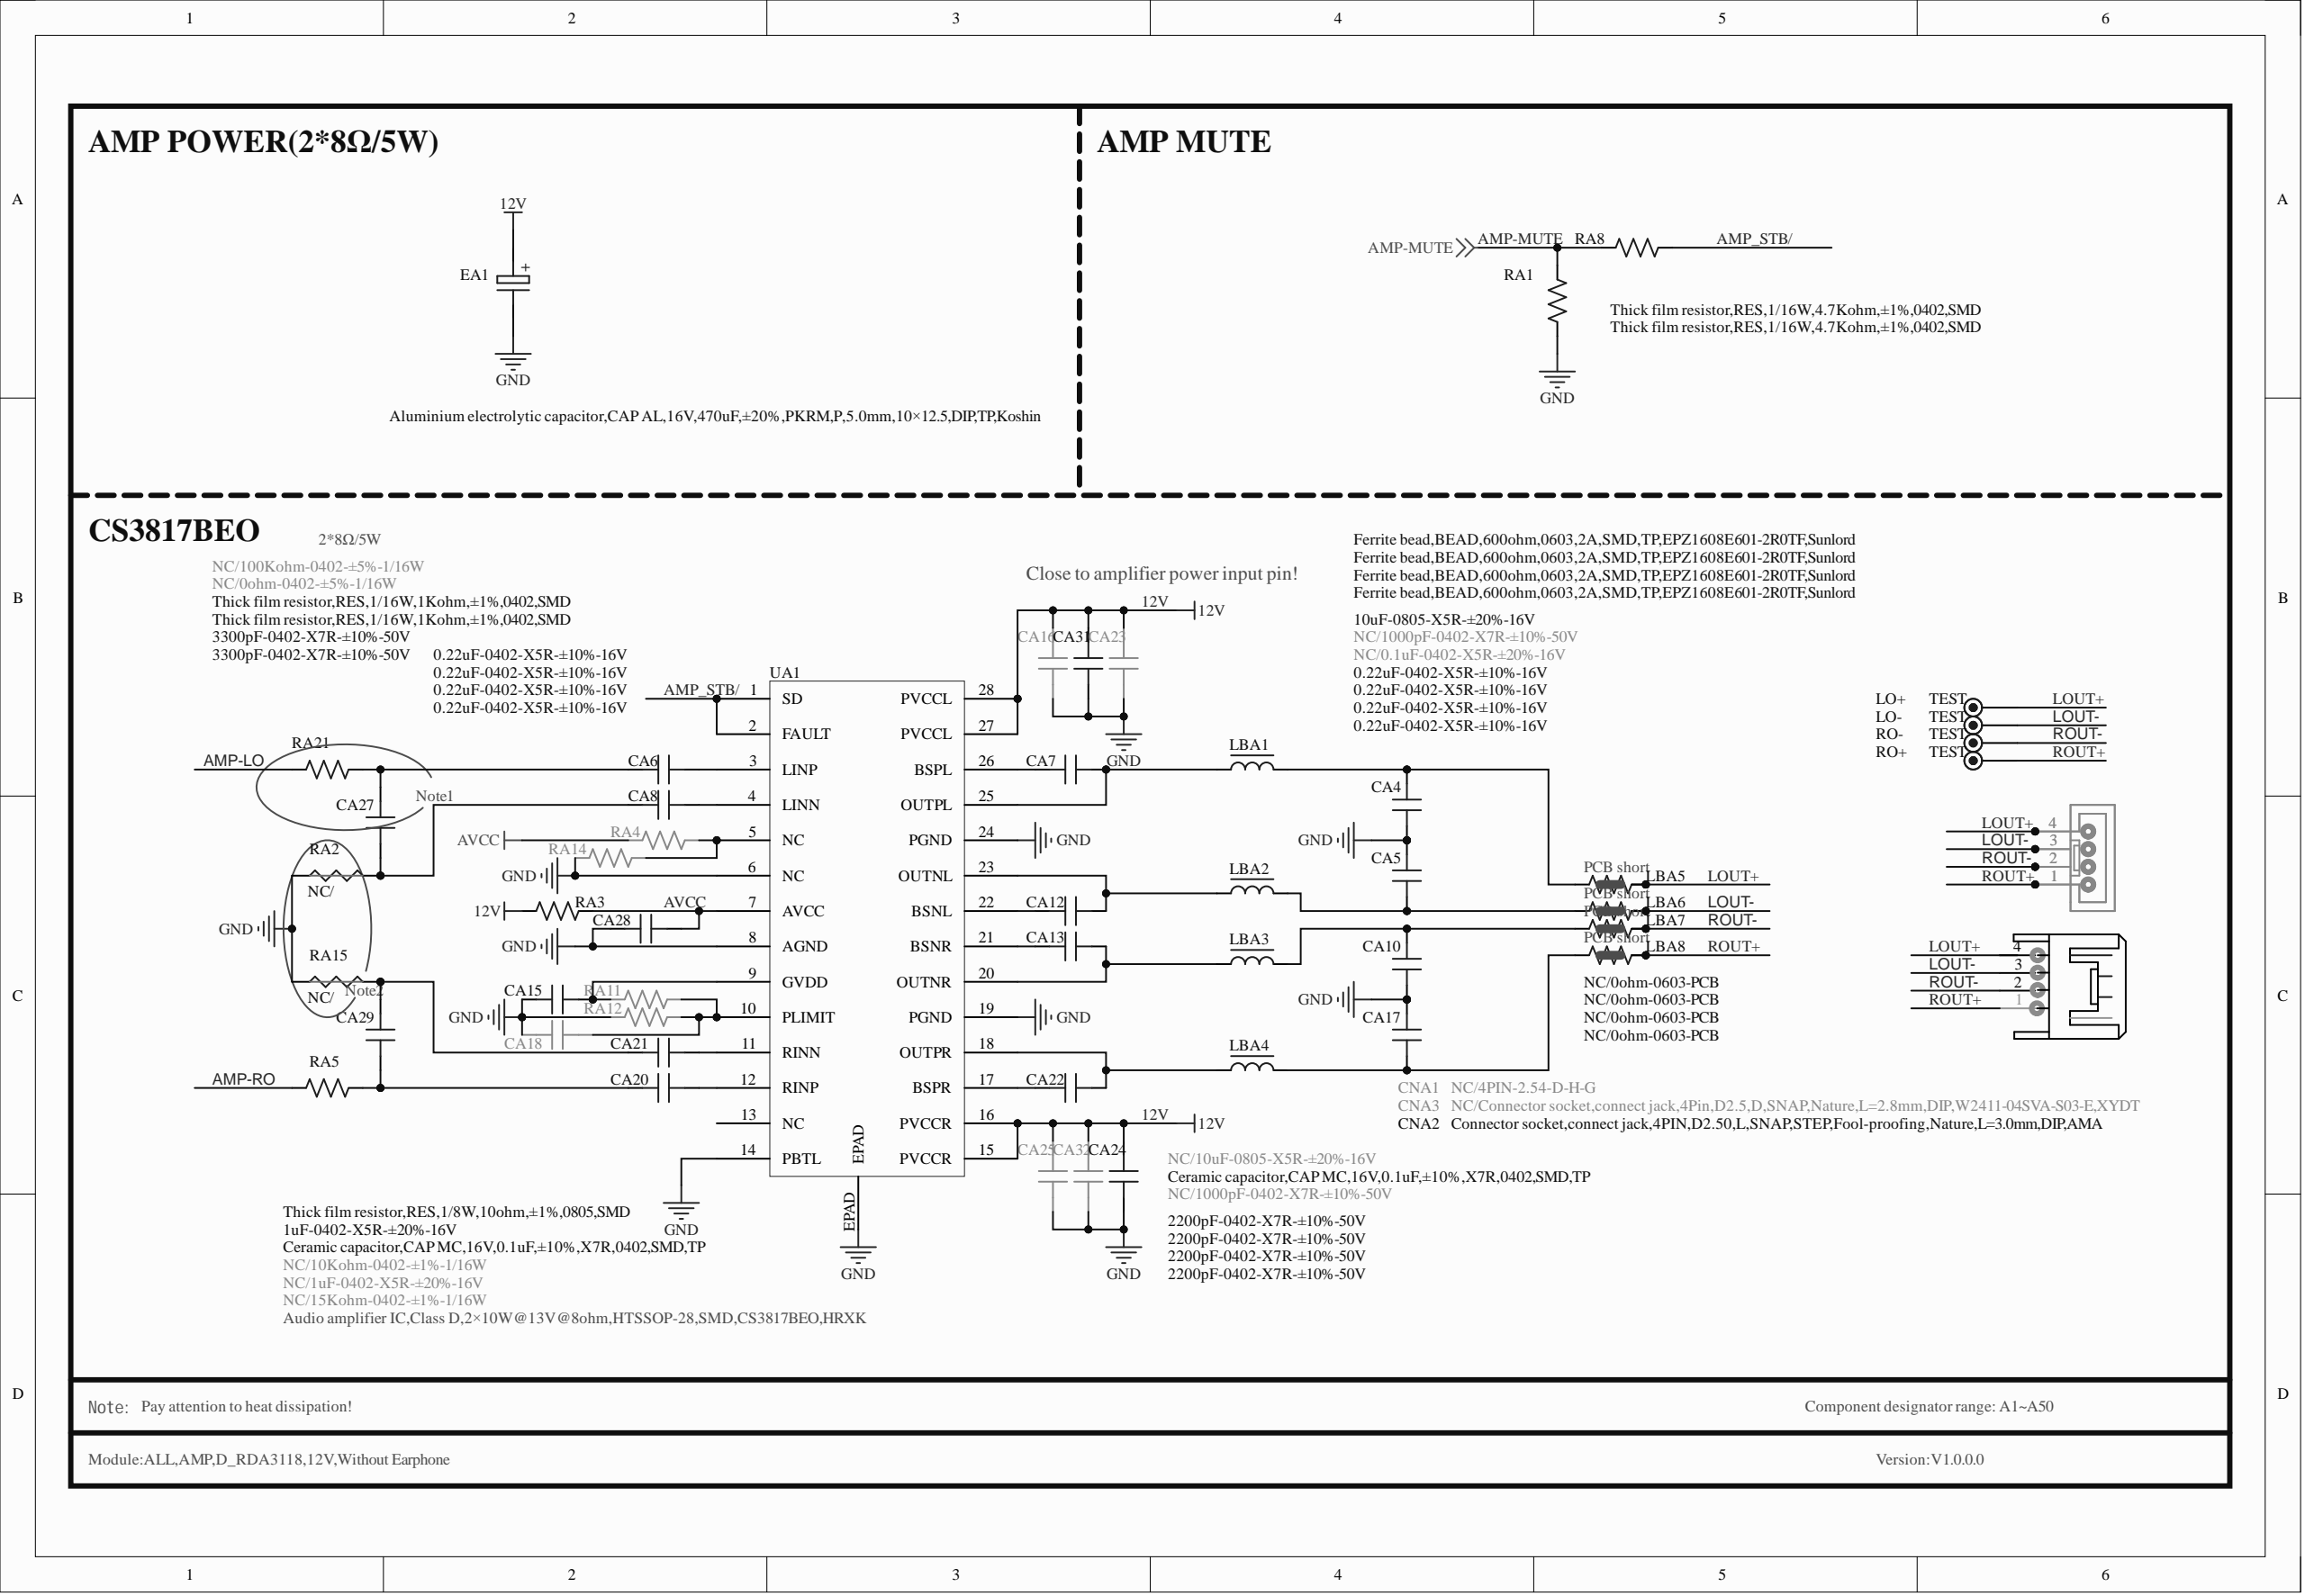Circuit board | Altium Designer | 719 parts | 352 nets | one sheet of the schematic
Parts on this sheet (reference | value | footprint):
CA4 | 2200pF-0402-X7R-±10%-50V | C0402
CA5 | 2200pF-0402-X7R-±10%-50V | C0402
CA6 | 0.22uF-0402-X5R-±10%-16V | C0402
CA7 | 0.22uF-0402-X5R-±10%-16V | C0402
CA8 | 0.22uF-0402-X5R-±10%-16V | C0402
CA10 | 2200pF-0402-X7R-±10%-50V | C0402
CA12 | 0.22uF-0402-X5R-±10%-16V | C0402
CA13 | 0.22uF-0402-X5R-±10%-16V | C0402
CA15 | Ceramic capacitor,CAP MC,16V,0.1uF,±10%,X7R,0402,SMD,TP | C0402
CA16 | NC/1000pF-0402-X7R-±10%-50V | C0402
CA17 | 2200pF-0402-X7R-±10%-50V | C0402
CA18 | NC/1uF-0402-X5R-±20%-16V | C0402
CA20 | 0.22uF-0402-X5R-±10%-16V | C0402
CA21 | 0.22uF-0402-X5R-±10%-16V | C0402
CA22 | 0.22uF-0402-X5R-±10%-16V | C0402
CA23 | NC/0.1uF-0402-X5R-±20%-16V | C0402
CA24 | Ceramic capacitor,CAP MC,16V,0.1uF,±10%,X7R,0402,SMD,TP | C0402
CA25 | NC/1000pF-0402-X7R-±10%-50V | C0402
CA27 | 3300pF-0402-X7R-±10%-50V | C0402
CA28 | 1uF-0402-X5R-±20%-16V | C0402
CA29 | 3300pF-0402-X7R-±10%-50V | C0402
CA31 | 10uF-0805-X5R-±20%-16V | C0805
CA32 | NC/10uF-0805-X5R-±20%-16V | C0805
CNA1 | NC/4PIN-2.54-D-H-G | SIP4/2.54D-1
CNA2 | Connector socket,connect jack,4PIN,D2.50,L,SNAP,STEP,Fool-proofing,Nature,L=3.0mm,DIP,AMA | SIP4H/2.5D-7
CNA3 | NC/Connector socket,connect jack,4Pin,D2.5,D,SNAP,Nature,L=2.8mm,DIP,W2411-04SVA-S03-E,XYDT | SIP4/2.5D-2
EA1 | Aluminium electrolytic capacitor,CAP AL,16V,470uF,±20%,PKRM,P,5.0mm,10×12.5,DIP,TP,Koshin | EC(10*12.5)-V-5
LBA1 | Ferrite bead,BEAD,600ohm,0603,2A,SMD,TP,EPZ1608E601-2R0TF,Sunlord | L0603
LBA2 | Ferrite bead,BEAD,600ohm,0603,2A,SMD,TP,EPZ1608E601-2R0TF,Sunlord | L0603
LBA3 | Ferrite bead,BEAD,600ohm,0603,2A,SMD,TP,EPZ1608E601-2R0TF,Sunlord | L0603
LBA4 | Ferrite bead,BEAD,600ohm,0603,2A,SMD,TP,EPZ1608E601-2R0TF,Sunlord | L0603
LO+ | TEST | TP
LO- | TEST | TP
RA1 | Thick film resistor,RES,1/16W,4.7Kohm,±1%,0402,SMD | R0402
RA2 | NC/ | GND
RA3 | Thick film resistor,RES,1/8W,10ohm,±1%,0805,SMD | R0805
RA4 | NC/100Kohm-0402-±5%-1/16W | R0402
RA5 | Thick film resistor,RES,1/16W,1Kohm,±1%,0402,SMD | R0402
RA8 | Thick film resistor,RES,1/16W,4.7Kohm,±1%,0402,SMD | R0402
RA11 | NC/10Kohm-0402-±1%-1/16W | R0402
RA12 | NC/15Kohm-0402-±1%-1/16W | R0402
RA14 | NC/0ohm-0402-±5%-1/16W | R0402
RA15 | NC/ | GND
RA21 | Thick film resistor,RES,1/16W,1Kohm,±1%,0402,SMD | R0402
RO+ | TEST | TP
RO- | TEST | TP
UA1 | Audio amplifier IC,Class D,2×10W@13V@8ohm,HTSSOP-28,SMD,CS3817BEO,HRXK | SSOP28/0.65-5
Nets of these parts (net: part-pin ...):
ROUT-: CNA1-2 CNA2-2 CNA3-2 RO--1
ROUT+: CNA1-1 CNA2-1 CNA3-1 RO+-1
NetRA4_1: RA4-1 RA14-2 UA1-5
NetCA22_2: CA22-2 LBA4-1 UA1-18
NetCA22_1: CA22-1 UA1-17
NetCA21_2: CA21-2 CA29-2 RA15-JP_1K
NetCA21_1: CA21-1 UA1-11
NetCA20_2: CA20-2 CA29-1 RA5-2
NetCA20_1: CA20-1 UA1-12
NetCA18_1: CA18-1 RA11-1 RA12-1 UA1-10
NetCA17_2: CA17-2 LBA4-2
NetCA15_1: CA15-1 RA11-2 UA1-9
NetCA13_2: CA13-2 LBA3-1 UA1-20
NetCA13_1: CA13-1 UA1-21
NetCA12_2: CA12-2 LBA2-1 UA1-23
NetCA12_1: CA12-1 UA1-22
NetCA10_1: CA10-1 LBA3-2
NetCA8_2: CA8-2 CA27-2 RA2-JP_1K
NetCA8_1: CA8-1 UA1-4
NetCA7_2: CA7-2 LBA1-1 UA1-25
NetCA7_1: CA7-1 UA1-26
NetCA6_2: CA6-2 CA27-1 RA21-2
NetCA6_1: CA6-1 UA1-3
NetCA5_1: CA5-1 LBA2-2
NetCA4_1: CA4-1 LBA1-2
LOUT-: CNA1-3 CNA2-3 CNA3-3 LO--1
LOUT+: CNA1-4 CNA2-4 CNA3-4 LO+-1
GND: CA4-2 CA5-2 CA10-2 CA15-2 CA16-1 CA17-1 CA18-2 CA23-1 CA24-1 CA25-1 CA28-1 CA31-1 CA32-1 EA1-2 RA1-1 RA2-JP_2K RA12-2 RA14-1 RA15-JP_2K UA1-6 UA1-8 UA1-14 UA1-19 UA1-24 UA1-EPAD
AVCC: CA28-2 RA3-2 RA4-2 UA1-7
AMP_STB/: RA8-2 UA1-1 UA1-2
AMP-RO: RA5-1
AMP-MUTE: RA1-2 RA8-1
AMP-LO: RA21-1
12V: CA16-2 CA23-2 CA24-2 CA25-2 CA31-2 CA32-2 EA1-1 RA3-1 UA1-15 UA1-16 UA1-27 UA1-28